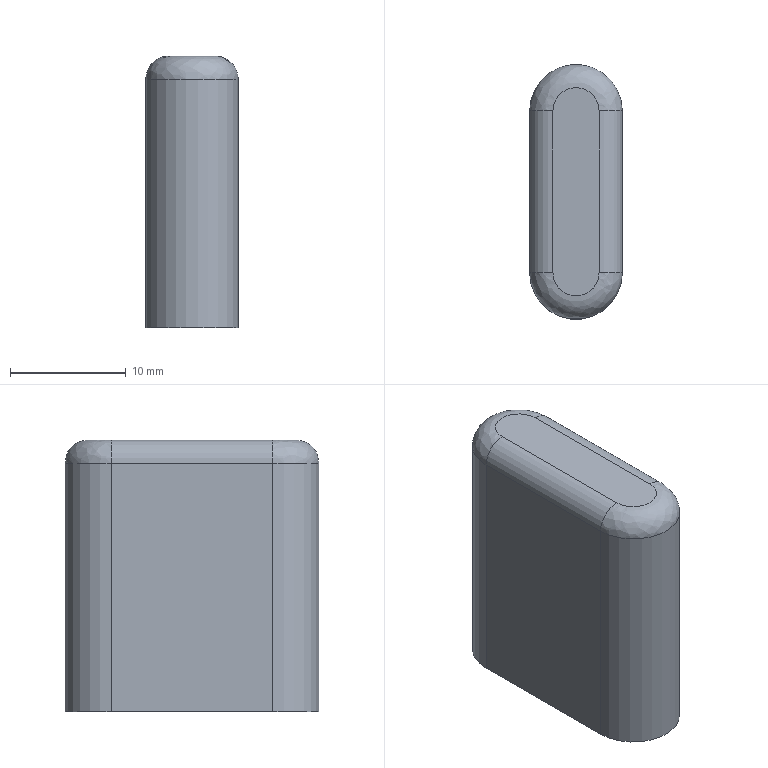Part | STEP file | Tube feed_id1790_x_t | 1 solid | 10 faces | box 8 x 22 x 23.5 mm | volume 3770 mm3 | plane 4 | cylinder 4 | spline 2 | commonest cylinder face diameters 4 x2 8 x2
STEP:
#1=CARTESIAN_POINT('',(0.,0.,0.));
#2=DIRECTION('',(0.,0.,1.));
#3=DIRECTION('',(1.,0.,0.));
#4=AXIS2_PLACEMENT_3D('',#1,#2,#3);
#5=CARTESIAN_POINT('',(17.,-36.964,-19.5));
#6=VERTEX_POINT('',#5);
#7=CARTESIAN_POINT('',(17.,-50.964,-19.5));
#8=VERTEX_POINT('',#7);
#9=CARTESIAN_POINT('',(17.,-32.964,-19.5));
#10=DIRECTION('',(0.,-1.,0.));
#11=VECTOR('',#10,1.);
#12=LINE('',#9,#11);
#13=CARTESIAN_POINT('',(25.,-32.964,-19.5));
#14=DIRECTION('',(0.,0.,-1.));
#15=DIRECTION('',(0.,-1.,0.));
#16=AXIS2_PLACEMENT_3D('',#13,#14,#15);
#17=PLANE('',#16);
#18=CARTESIAN_POINT('',(0.,8.));
#19=DIRECTION('',(1.,0.));
#20=VECTOR('',#19,1.);
#21=LINE('',#18,#20);
#22=(GEOMETRIC_REPRESENTATION_CONTEXT(2)PARAMETRIC_REPRESENTATION_CONTEXT()REPRESENTATION_CONTEXT('',''));
#23=DEFINITIONAL_REPRESENTATION('',(#21),#22);
#24=PCURVE('',#17,#23);
#25=CARTESIAN_POINT('',(17.,-32.964,-19.5));
#26=DIRECTION('',(1.,0.,0.));
#27=DIRECTION('',(0.,0.,-1.));
#28=AXIS2_PLACEMENT_3D('',#25,#26,#27);
#29=PLANE('',#28);
#30=CARTESIAN_POINT('',(0.,0.));
#31=DIRECTION('',(0.,-1.));
#32=VECTOR('',#31,1.);
#33=LINE('',#30,#32);
#34=(GEOMETRIC_REPRESENTATION_CONTEXT(2)PARAMETRIC_REPRESENTATION_CONTEXT()REPRESENTATION_CONTEXT('',''));
#35=DEFINITIONAL_REPRESENTATION('',(#33),#34);
#36=PCURVE('',#29,#35);
#37=SURFACE_CURVE('',#12,(#24,#36),.PCURVE_S1.);
#38=EDGE_CURVE('',#6,#8,#37,.T.);
#39=ORIENTED_EDGE('',*,*,#38,.F.);
#40=CARTESIAN_POINT('',(25.,-36.964,-19.5));
#41=VERTEX_POINT('',#40);
#42=CARTESIAN_POINT('',(21.,-36.964,-19.5));
#43=DIRECTION('',(0.,0.,1.));
#44=DIRECTION('',(0.,-1.,0.));
#45=AXIS2_PLACEMENT_3D('',#42,#43,#44);
#46=CIRCLE('',#45,4.);
#47=CARTESIAN_POINT('',(8.,4.));
#48=CARTESIAN_POINT('',(8.,-2.928));
#49=CARTESIAN_POINT('',(2.,0.5359));
#50=CARTESIAN_POINT('',(-4.,4.));
#51=CARTESIAN_POINT('',(2.,7.464));
#52=CARTESIAN_POINT('',(8.,10.928));
#53=CARTESIAN_POINT('',(8.,4.));
#54=(BOUNDED_CURVE()B_SPLINE_CURVE(2,(#47,#48,#49,#50,#51,#52,#53),.UNSPECIFIED.,.T.,.F.)B_SPLINE_CURVE_WITH_KNOTS((1,2,2,2,2,1),(-2.094,0.,2.094,4.189,6.283,8.378),.UNSPECIFIED.)CURVE()GEOMETRIC_REPRESENTATION_ITEM()RATIONAL_B_SPLINE_CURVE((1.,0.5,1.,0.5,1.,0.5,1.))REPRESENTATION_ITEM(''));
#55=(GEOMETRIC_REPRESENTATION_CONTEXT(2)PARAMETRIC_REPRESENTATION_CONTEXT()REPRESENTATION_CONTEXT('',''));
#56=DEFINITIONAL_REPRESENTATION('',(#54),#55);
#57=PCURVE('',#17,#56);
#58=CARTESIAN_POINT('',(21.,-36.964,-19.5));
#59=DIRECTION('',(0.,0.,-1.));
#60=DIRECTION('',(-1.,0.,0.));
#61=AXIS2_PLACEMENT_3D('',#58,#59,#60);
#62=CYLINDRICAL_SURFACE('',#61,4.);
#63=CARTESIAN_POINT('',(4.712,0.));
#64=DIRECTION('',(-1.,0.));
#65=VECTOR('',#64,1.);
#66=LINE('',#63,#65);
#67=(GEOMETRIC_REPRESENTATION_CONTEXT(2)PARAMETRIC_REPRESENTATION_CONTEXT()REPRESENTATION_CONTEXT('',''));
#68=DEFINITIONAL_REPRESENTATION('',(#66),#67);
#69=PCURVE('',#62,#68);
#70=SURFACE_CURVE('',#46,(#57,#69),.PCURVE_S1.);
#71=EDGE_CURVE('',#41,#6,#70,.T.);
#72=ORIENTED_EDGE('',*,*,#71,.F.);
#73=CARTESIAN_POINT('',(25.,-50.964,-19.5));
#74=VERTEX_POINT('',#73);
#75=CARTESIAN_POINT('',(25.,-32.964,-19.5));
#76=DIRECTION('',(0.,-1.,0.));
#77=VECTOR('',#76,1.);
#78=LINE('',#75,#77);
#79=CARTESIAN_POINT('',(0.,0.));
#80=DIRECTION('',(1.,0.));
#81=VECTOR('',#80,1.);
#82=LINE('',#79,#81);
#83=(GEOMETRIC_REPRESENTATION_CONTEXT(2)PARAMETRIC_REPRESENTATION_CONTEXT()REPRESENTATION_CONTEXT('',''));
#84=DEFINITIONAL_REPRESENTATION('',(#82),#83);
#85=PCURVE('',#17,#84);
#86=CARTESIAN_POINT('',(25.,-32.964,-19.5));
#87=DIRECTION('',(1.,0.,0.));
#88=DIRECTION('',(0.,0.,-1.));
#89=AXIS2_PLACEMENT_3D('',#86,#87,#88);
#90=PLANE('',#89);
#91=CARTESIAN_POINT('',(0.,0.));
#92=DIRECTION('',(0.,-1.));
#93=VECTOR('',#92,1.);
#94=LINE('',#91,#93);
#95=(GEOMETRIC_REPRESENTATION_CONTEXT(2)PARAMETRIC_REPRESENTATION_CONTEXT()REPRESENTATION_CONTEXT('',''));
#96=DEFINITIONAL_REPRESENTATION('',(#94),#95);
#97=PCURVE('',#90,#96);
#98=SURFACE_CURVE('',#78,(#85,#97),.PCURVE_S1.);
#99=EDGE_CURVE('',#41,#74,#98,.T.);
#100=ORIENTED_EDGE('',*,*,#99,.T.);
#101=CARTESIAN_POINT('',(21.,-50.964,-19.5));
#102=DIRECTION('',(0.,0.,1.));
#103=DIRECTION('',(0.,-1.,0.));
#104=AXIS2_PLACEMENT_3D('',#101,#102,#103);
#105=CIRCLE('',#104,4.);
#106=CARTESIAN_POINT('',(22.,4.));
#107=CARTESIAN_POINT('',(22.,-2.928));
#108=CARTESIAN_POINT('',(16.,0.5359));
#109=CARTESIAN_POINT('',(10.,4.));
#110=CARTESIAN_POINT('',(16.,7.464));
#111=CARTESIAN_POINT('',(22.,10.928));
#112=CARTESIAN_POINT('',(22.,4.));
#113=(BOUNDED_CURVE()B_SPLINE_CURVE(2,(#106,#107,#108,#109,#110,#111,#112),.UNSPECIFIED.,.T.,.F.)B_SPLINE_CURVE_WITH_KNOTS((1,2,2,2,2,1),(-2.094,0.,2.094,4.189,6.283,8.378),.UNSPECIFIED.)CURVE()GEOMETRIC_REPRESENTATION_ITEM()RATIONAL_B_SPLINE_CURVE((1.,0.5,1.,0.5,1.,0.5,1.))REPRESENTATION_ITEM(''));
#114=(GEOMETRIC_REPRESENTATION_CONTEXT(2)PARAMETRIC_REPRESENTATION_CONTEXT()REPRESENTATION_CONTEXT('',''));
#115=DEFINITIONAL_REPRESENTATION('',(#113),#114);
#116=PCURVE('',#17,#115);
#117=CARTESIAN_POINT('',(21.,-50.964,-19.5));
#118=DIRECTION('',(0.,0.,1.));
#119=DIRECTION('',(1.,0.,0.));
#120=AXIS2_PLACEMENT_3D('',#117,#118,#119);
#121=CYLINDRICAL_SURFACE('',#120,4.);
#122=CARTESIAN_POINT('',(-1.571,0.));
#123=DIRECTION('',(1.,0.));
#124=VECTOR('',#123,1.);
#125=LINE('',#122,#124);
#126=(GEOMETRIC_REPRESENTATION_CONTEXT(2)PARAMETRIC_REPRESENTATION_CONTEXT()REPRESENTATION_CONTEXT('',''));
#127=DEFINITIONAL_REPRESENTATION('',(#125),#126);
#128=PCURVE('',#121,#127);
#129=SURFACE_CURVE('',#105,(#116,#128),.PCURVE_S1.);
#130=EDGE_CURVE('',#8,#74,#129,.T.);
#131=ORIENTED_EDGE('',*,*,#130,.F.);
#132=EDGE_LOOP('',(#39,#72,#100,#131));
#133=FACE_BOUND('',#132,.T.);
#134=ADVANCED_FACE('',(#133),#17,.T.);
#135=CARTESIAN_POINT('',(19.,-50.964,4.));
#136=VERTEX_POINT('',#135);
#137=CARTESIAN_POINT('',(23.,-50.964,4.));
#138=VERTEX_POINT('',#137);
#139=CARTESIAN_POINT('',(21.,-50.964,4.));
#140=DIRECTION('',(0.,0.,1.));
#141=DIRECTION('',(0.,1.,0.));
#142=AXIS2_PLACEMENT_3D('',#139,#140,#141);
#143=CIRCLE('',#142,2.);
#144=CARTESIAN_POINT('',(25.,-32.964,4.));
#145=DIRECTION('',(0.,0.,-1.));
#146=DIRECTION('',(0.,-1.,0.));
#147=AXIS2_PLACEMENT_3D('',#144,#145,#146);
#148=PLANE('',#147);
#149=CARTESIAN_POINT('',(16.,4.));
#150=CARTESIAN_POINT('',(16.,7.464));
#151=CARTESIAN_POINT('',(19.,5.732));
#152=CARTESIAN_POINT('',(22.,4.));
#153=CARTESIAN_POINT('',(19.,2.268));
#154=CARTESIAN_POINT('',(16.,0.5359));
#155=CARTESIAN_POINT('',(16.,4.));
#156=(BOUNDED_CURVE()B_SPLINE_CURVE(2,(#149,#150,#151,#152,#153,#154,#155),.UNSPECIFIED.,.T.,.F.)B_SPLINE_CURVE_WITH_KNOTS((1,2,2,2,2,1),(-2.094,0.,2.094,4.189,6.283,8.378),.UNSPECIFIED.)CURVE()GEOMETRIC_REPRESENTATION_ITEM()RATIONAL_B_SPLINE_CURVE((1.,0.5,1.,0.5,1.,0.5,1.))REPRESENTATION_ITEM(''));
#157=(GEOMETRIC_REPRESENTATION_CONTEXT(2)PARAMETRIC_REPRESENTATION_CONTEXT()REPRESENTATION_CONTEXT('',''));
#158=DEFINITIONAL_REPRESENTATION('',(#156),#157);
#159=PCURVE('',#148,#158);
#160=CARTESIAN_POINT('',(25.,-50.964,2.));
#161=CARTESIAN_POINT('',(25.,-58.964,2.));
#162=CARTESIAN_POINT('',(17.,-58.964,2.));
#163=CARTESIAN_POINT('',(17.,-50.964,2.));
#164=CARTESIAN_POINT('',(25.,-50.964,3.172));
#165=CARTESIAN_POINT('',(25.,-58.964,3.172));
#166=CARTESIAN_POINT('',(17.,-58.964,3.172));
#167=CARTESIAN_POINT('',(17.,-50.964,3.172));
#168=CARTESIAN_POINT('',(24.172,-50.964,4.));
#169=CARTESIAN_POINT('',(24.172,-57.308,4.));
#170=CARTESIAN_POINT('',(17.828,-57.308,4.));
#171=CARTESIAN_POINT('',(17.828,-50.964,4.));
#172=CARTESIAN_POINT('',(23.,-50.964,4.));
#173=CARTESIAN_POINT('',(23.,-54.964,4.));
#174=CARTESIAN_POINT('',(19.,-54.964,4.));
#175=CARTESIAN_POINT('',(19.,-50.964,4.));
#176=(BOUNDED_SURFACE()B_SPLINE_SURFACE(3,3,((#160,#161,#162,#163),(#164,#165,#166,#167),(#168,#169,#170,#171),(#172,#173,#174,#175)),.UNSPECIFIED.,.F.,.F.,.F.)B_SPLINE_SURFACE_WITH_KNOTS((4,4),(4,4),(0.,1.),(0.,1.),.PIECEWISE_BEZIER_KNOTS.)GEOMETRIC_REPRESENTATION_ITEM()RATIONAL_B_SPLINE_SURFACE(((1.,0.3333,0.3333,1.),(0.8047,0.2682,0.2682,0.8047),(0.8047,0.2682,0.2682,0.8047),(1.,0.3333,0.3333,1.)))REPRESENTATION_ITEM('')SURFACE());
#177=CARTESIAN_POINT('',(1.,1.));
#178=CARTESIAN_POINT('',(1.,0.9763));
#179=CARTESIAN_POINT('',(1.,0.9319));
#180=CARTESIAN_POINT('',(1.,0.8733));
#181=CARTESIAN_POINT('',(1.,0.8206));
#182=CARTESIAN_POINT('',(1.,0.7724));
#183=CARTESIAN_POINT('',(1.,0.7279));
#184=CARTESIAN_POINT('',(1.,0.6861));
#185=CARTESIAN_POINT('',(1.,0.6465));
#186=CARTESIAN_POINT('',(1.,0.6086));
#187=CARTESIAN_POINT('',(1.,0.5718));
#188=CARTESIAN_POINT('',(1.,0.5357));
#189=CARTESIAN_POINT('',(1.,0.5));
#190=CARTESIAN_POINT('',(1.,0.4643));
#191=CARTESIAN_POINT('',(1.,0.4282));
#192=CARTESIAN_POINT('',(1.,0.3914));
#193=CARTESIAN_POINT('',(1.,0.3535));
#194=CARTESIAN_POINT('',(1.,0.3139));
#195=CARTESIAN_POINT('',(1.,0.2721));
#196=CARTESIAN_POINT('',(1.,0.2276));
#197=CARTESIAN_POINT('',(1.,0.1794));
#198=CARTESIAN_POINT('',(1.,0.1267));
#199=CARTESIAN_POINT('',(1.,0.06805));
#200=CARTESIAN_POINT('',(1.,0.02375));
#201=CARTESIAN_POINT('',(1.,0.));
#202=B_SPLINE_CURVE_WITH_KNOTS('',3,(#177,#178,#179,#180,#181,#182,#183,#184,#185,#186,#187,#188,#189,#190,#191,#192,#193,#194,#195,#196,#197,#198,#199,#200,#201),.UNSPECIFIED.,.F.,.F.,(4,1,1,1,1,1,1,1,1,1,1,1,1,1,1,1,1,1,1,1,1,1,4),(1.571,1.714,1.856,1.999,2.142,2.285,2.428,2.57,2.713,2.856,2.999,3.142,3.284,3.427,3.57,3.713,3.856,3.998,4.141,4.284,4.427,4.57,4.712),.QUASI_UNIFORM_KNOTS.);
#203=(GEOMETRIC_REPRESENTATION_CONTEXT(2)PARAMETRIC_REPRESENTATION_CONTEXT()REPRESENTATION_CONTEXT('',''));
#204=DEFINITIONAL_REPRESENTATION('',(#202),#203);
#205=PCURVE('',#176,#204);
#206=SURFACE_CURVE('',#143,(#159,#205),.PCURVE_S1.);
#207=EDGE_CURVE('',#136,#138,#206,.T.);
#208=ORIENTED_EDGE('',*,*,#207,.T.);
#209=CARTESIAN_POINT('',(23.,-36.964,4.));
#210=VERTEX_POINT('',#209);
#211=CARTESIAN_POINT('',(23.,-32.964,4.));
#212=DIRECTION('',(0.,1.,0.));
#213=VECTOR('',#212,1.);
#214=LINE('',#211,#213);
#215=CARTESIAN_POINT('',(0.,2.));
#216=DIRECTION('',(-1.,0.));
#217=VECTOR('',#216,1.);
#218=LINE('',#215,#217);
#219=(GEOMETRIC_REPRESENTATION_CONTEXT(2)PARAMETRIC_REPRESENTATION_CONTEXT()REPRESENTATION_CONTEXT('',''));
#220=DEFINITIONAL_REPRESENTATION('',(#218),#219);
#221=PCURVE('',#148,#220);
#222=CARTESIAN_POINT('',(23.,-32.964,2.));
#223=DIRECTION('',(0.,-1.,0.));
#224=DIRECTION('',(1.,0.,0.));
#225=AXIS2_PLACEMENT_3D('',#222,#223,#224);
#226=CYLINDRICAL_SURFACE('',#225,2.);
#227=CARTESIAN_POINT('',(1.571,0.));
#228=DIRECTION('',(0.,-1.));
#229=VECTOR('',#228,1.);
#230=LINE('',#227,#229);
#231=(GEOMETRIC_REPRESENTATION_CONTEXT(2)PARAMETRIC_REPRESENTATION_CONTEXT()REPRESENTATION_CONTEXT('',''));
#232=DEFINITIONAL_REPRESENTATION('',(#230),#231);
#233=PCURVE('',#226,#232);
#234=SURFACE_CURVE('',#214,(#221,#233),.PCURVE_S1.);
#235=EDGE_CURVE('',#138,#210,#234,.T.);
#236=ORIENTED_EDGE('',*,*,#235,.T.);
#237=CARTESIAN_POINT('',(19.,-36.964,4.));
#238=VERTEX_POINT('',#237);
#239=CARTESIAN_POINT('',(21.,-36.964,4.));
#240=DIRECTION('',(0.,0.,1.));
#241=DIRECTION('',(0.,1.,0.));
#242=AXIS2_PLACEMENT_3D('',#239,#240,#241);
#243=CIRCLE('',#242,2.);
#244=CARTESIAN_POINT('',(2.,4.));
#245=CARTESIAN_POINT('',(2.,7.464));
#246=CARTESIAN_POINT('',(5.,5.732));
#247=CARTESIAN_POINT('',(8.,4.));
#248=CARTESIAN_POINT('',(5.,2.268));
#249=CARTESIAN_POINT('',(2.,0.5359));
#250=CARTESIAN_POINT('',(2.,4.));
#251=(BOUNDED_CURVE()B_SPLINE_CURVE(2,(#244,#245,#246,#247,#248,#249,#250),.UNSPECIFIED.,.T.,.F.)B_SPLINE_CURVE_WITH_KNOTS((1,2,2,2,2,1),(-2.094,0.,2.094,4.189,6.283,8.378),.UNSPECIFIED.)CURVE()GEOMETRIC_REPRESENTATION_ITEM()RATIONAL_B_SPLINE_CURVE((1.,0.5,1.,0.5,1.,0.5,1.))REPRESENTATION_ITEM(''));
#252=(GEOMETRIC_REPRESENTATION_CONTEXT(2)PARAMETRIC_REPRESENTATION_CONTEXT()REPRESENTATION_CONTEXT('',''));
#253=DEFINITIONAL_REPRESENTATION('',(#251),#252);
#254=PCURVE('',#148,#253);
#255=CARTESIAN_POINT('',(17.,-36.964,2.));
#256=CARTESIAN_POINT('',(17.,-28.964,2.));
#257=CARTESIAN_POINT('',(25.,-28.964,2.));
#258=CARTESIAN_POINT('',(25.,-36.964,2.));
#259=CARTESIAN_POINT('',(17.,-36.964,3.172));
#260=CARTESIAN_POINT('',(17.,-28.964,3.172));
#261=CARTESIAN_POINT('',(25.,-28.964,3.172));
#262=CARTESIAN_POINT('',(25.,-36.964,3.172));
#263=CARTESIAN_POINT('',(17.828,-36.964,4.));
#264=CARTESIAN_POINT('',(17.828,-30.621,4.));
#265=CARTESIAN_POINT('',(24.172,-30.621,4.));
#266=CARTESIAN_POINT('',(24.172,-36.964,4.));
#267=CARTESIAN_POINT('',(19.,-36.964,4.));
#268=CARTESIAN_POINT('',(19.,-32.964,4.));
#269=CARTESIAN_POINT('',(23.,-32.964,4.));
#270=CARTESIAN_POINT('',(23.,-36.964,4.));
#271=(BOUNDED_SURFACE()B_SPLINE_SURFACE(3,3,((#255,#256,#257,#258),(#259,#260,#261,#262),(#263,#264,#265,#266),(#267,#268,#269,#270)),.UNSPECIFIED.,.F.,.F.,.F.)B_SPLINE_SURFACE_WITH_KNOTS((4,4),(4,4),(0.,1.),(0.,1.),.PIECEWISE_BEZIER_KNOTS.)GEOMETRIC_REPRESENTATION_ITEM()RATIONAL_B_SPLINE_SURFACE(((1.,0.3333,0.3333,1.),(0.8047,0.2682,0.2682,0.8047),(0.8047,0.2682,0.2682,0.8047),(1.,0.3333,0.3333,1.)))REPRESENTATION_ITEM('')SURFACE());
#272=CARTESIAN_POINT('',(1.,1.));
#273=CARTESIAN_POINT('',(1.,0.9763));
#274=CARTESIAN_POINT('',(1.,0.9319));
#275=CARTESIAN_POINT('',(1.,0.8733));
#276=CARTESIAN_POINT('',(1.,0.8206));
#277=CARTESIAN_POINT('',(1.,0.7724));
#278=CARTESIAN_POINT('',(1.,0.7279));
#279=CARTESIAN_POINT('',(1.,0.6861));
#280=CARTESIAN_POINT('',(1.,0.6465));
#281=CARTESIAN_POINT('',(1.,0.6086));
#282=CARTESIAN_POINT('',(1.,0.5718));
#283=CARTESIAN_POINT('',(1.,0.5357));
#284=CARTESIAN_POINT('',(1.,0.5));
#285=CARTESIAN_POINT('',(1.,0.4643));
#286=CARTESIAN_POINT('',(1.,0.4282));
#287=CARTESIAN_POINT('',(1.,0.3914));
#288=CARTESIAN_POINT('',(1.,0.3535));
#289=CARTESIAN_POINT('',(1.,0.3139));
#290=CARTESIAN_POINT('',(1.,0.2721));
#291=CARTESIAN_POINT('',(1.,0.2276));
#292=CARTESIAN_POINT('',(1.,0.1794));
#293=CARTESIAN_POINT('',(1.,0.1267));
#294=CARTESIAN_POINT('',(1.,0.06805));
#295=CARTESIAN_POINT('',(1.,0.02375));
#296=CARTESIAN_POINT('',(1.,0.));
#297=B_SPLINE_CURVE_WITH_KNOTS('',3,(#272,#273,#274,#275,#276,#277,#278,#279,#280,#281,#282,#283,#284,#285,#286,#287,#288,#289,#290,#291,#292,#293,#294,#295,#296),.UNSPECIFIED.,.F.,.F.,(4,1,1,1,1,1,1,1,1,1,1,1,1,1,1,1,1,1,1,1,1,1,4),(4.712,4.855,4.998,5.141,5.284,5.426,5.569,5.712,5.855,5.998,6.14,6.283,6.426,6.569,6.712,6.854,6.997,7.14,7.283,7.426,7.568,7.711,7.854),.QUASI_UNIFORM_KNOTS.);
#298=(GEOMETRIC_REPRESENTATION_CONTEXT(2)PARAMETRIC_REPRESENTATION_CONTEXT()REPRESENTATION_CONTEXT('',''));
#299=DEFINITIONAL_REPRESENTATION('',(#297),#298);
#300=PCURVE('',#271,#299);
#301=SURFACE_CURVE('',#243,(#254,#300),.PCURVE_S1.);
#302=EDGE_CURVE('',#210,#238,#301,.T.);
#303=ORIENTED_EDGE('',*,*,#302,.T.);
#304=CARTESIAN_POINT('',(19.,-50.964,4.));
#305=DIRECTION('',(0.,-1.,0.));
#306=VECTOR('',#305,1.);
#307=LINE('',#304,#306);
#308=CARTESIAN_POINT('',(18.,6.));
#309=DIRECTION('',(1.,0.));
#310=VECTOR('',#309,1.);
#311=LINE('',#308,#310);
#312=(GEOMETRIC_REPRESENTATION_CONTEXT(2)PARAMETRIC_REPRESENTATION_CONTEXT()REPRESENTATION_CONTEXT('',''));
#313=DEFINITIONAL_REPRESENTATION('',(#311),#312);
#314=PCURVE('',#148,#313);
#315=CARTESIAN_POINT('',(19.,-32.964,2.));
#316=DIRECTION('',(0.,1.,0.));
#317=DIRECTION('',(-1.,0.,0.));
#318=AXIS2_PLACEMENT_3D('',#315,#316,#317);
#319=CYLINDRICAL_SURFACE('',#318,2.);
#320=CARTESIAN_POINT('',(1.571,-18.));
#321=DIRECTION('',(0.,-1.));
#322=VECTOR('',#321,1.);
#323=LINE('',#320,#322);
#324=(GEOMETRIC_REPRESENTATION_CONTEXT(2)PARAMETRIC_REPRESENTATION_CONTEXT()REPRESENTATION_CONTEXT('',''));
#325=DEFINITIONAL_REPRESENTATION('',(#323),#324);
#326=PCURVE('',#319,#325);
#327=SURFACE_CURVE('',#307,(#314,#326),.PCURVE_S1.);
#328=EDGE_CURVE('',#238,#136,#327,.T.);
#329=ORIENTED_EDGE('',*,*,#328,.T.);
#330=EDGE_LOOP('',(#208,#236,#303,#329));
#331=FACE_BOUND('',#330,.T.);
#332=ADVANCED_FACE('',(#331),#148,.F.);
#333=CARTESIAN_POINT('',(17.,-50.964,2.));
#334=VERTEX_POINT('',#333);
#335=CARTESIAN_POINT('',(17.,-50.964,-19.5));
#336=DIRECTION('',(0.,0.,-1.));
#337=VECTOR('',#336,1.);
#338=LINE('',#335,#337);
#339=CARTESIAN_POINT('',(0.,-18.));
#340=DIRECTION('',(1.,0.));
#341=VECTOR('',#340,1.);
#342=LINE('',#339,#341);
#343=(GEOMETRIC_REPRESENTATION_CONTEXT(2)PARAMETRIC_REPRESENTATION_CONTEXT()REPRESENTATION_CONTEXT('',''));
#344=DEFINITIONAL_REPRESENTATION('',(#342),#343);
#345=PCURVE('',#29,#344);
#346=CARTESIAN_POINT('',(3.142,0.));
#347=DIRECTION('',(0.,-1.));
#348=VECTOR('',#347,1.);
#349=LINE('',#346,#348);
#350=(GEOMETRIC_REPRESENTATION_CONTEXT(2)PARAMETRIC_REPRESENTATION_CONTEXT()REPRESENTATION_CONTEXT('',''));
#351=DEFINITIONAL_REPRESENTATION('',(#349),#350);
#352=PCURVE('',#121,#351);
#353=SURFACE_CURVE('',#338,(#345,#352),.PCURVE_S1.);
#354=EDGE_CURVE('',#334,#8,#353,.T.);
#355=ORIENTED_EDGE('',*,*,#354,.F.);
#356=CARTESIAN_POINT('',(17.,-36.964,2.));
#357=VERTEX_POINT('',#356);
#358=CARTESIAN_POINT('',(17.,-36.964,2.));
#359=DIRECTION('',(0.,1.,0.));
#360=VECTOR('',#359,1.);
#361=LINE('',#358,#360);
#362=CARTESIAN_POINT('',(-21.5,-4.));
#363=DIRECTION('',(0.,1.));
#364=VECTOR('',#363,1.);
#365=LINE('',#362,#364);
#366=(GEOMETRIC_REPRESENTATION_CONTEXT(2)PARAMETRIC_REPRESENTATION_CONTEXT()REPRESENTATION_CONTEXT('',''));
#367=DEFINITIONAL_REPRESENTATION('',(#365),#366);
#368=PCURVE('',#29,#367);
#369=CARTESIAN_POINT('',(0.,-4.));
#370=DIRECTION('',(0.,1.));
#371=VECTOR('',#370,1.);
#372=LINE('',#369,#371);
#373=(GEOMETRIC_REPRESENTATION_CONTEXT(2)PARAMETRIC_REPRESENTATION_CONTEXT()REPRESENTATION_CONTEXT('',''));
#374=DEFINITIONAL_REPRESENTATION('',(#372),#373);
#375=PCURVE('',#319,#374);
#376=SURFACE_CURVE('',#361,(#368,#375),.PCURVE_S1.);
#377=EDGE_CURVE('',#334,#357,#376,.T.);
#378=ORIENTED_EDGE('',*,*,#377,.T.);
#379=CARTESIAN_POINT('',(17.,-36.964,4.));
#380=DIRECTION('',(0.,0.,1.));
#381=VECTOR('',#380,1.);
#382=LINE('',#379,#381);
#383=CARTESIAN_POINT('',(-23.5,-4.));
#384=DIRECTION('',(-1.,0.));
#385=VECTOR('',#384,1.);
#386=LINE('',#383,#385);
#387=(GEOMETRIC_REPRESENTATION_CONTEXT(2)PARAMETRIC_REPRESENTATION_CONTEXT()REPRESENTATION_CONTEXT('',''));
#388=DEFINITIONAL_REPRESENTATION('',(#386),#387);
#389=PCURVE('',#29,#388);
#390=CARTESIAN_POINT('',(0.,-23.5));
#391=DIRECTION('',(0.,-1.));
#392=VECTOR('',#391,1.);
#393=LINE('',#390,#392);
#394=(GEOMETRIC_REPRESENTATION_CONTEXT(2)PARAMETRIC_REPRESENTATION_CONTEXT()REPRESENTATION_CONTEXT('',''));
#395=DEFINITIONAL_REPRESENTATION('',(#393),#394);
#396=PCURVE('',#62,#395);
#397=SURFACE_CURVE('',#382,(#389,#396),.PCURVE_S1.);
#398=EDGE_CURVE('',#6,#357,#397,.T.);
#399=ORIENTED_EDGE('',*,*,#398,.F.);
#400=ORIENTED_EDGE('',*,*,#38,.T.);
#401=EDGE_LOOP('',(#355,#378,#399,#400));
#402=FACE_BOUND('',#401,.T.);
#403=ADVANCED_FACE('',(#402),#29,.F.);
#404=CARTESIAN_POINT('',(25.,-36.964,2.));
#405=VERTEX_POINT('',#404);
#406=CARTESIAN_POINT('',(25.,-36.964,-19.5));
#407=DIRECTION('',(0.,0.,-1.));
#408=VECTOR('',#407,1.);
#409=LINE('',#406,#408);
#410=CARTESIAN_POINT('',(0.,-4.));
#411=DIRECTION('',(1.,0.));
#412=VECTOR('',#411,1.);
#413=LINE('',#410,#412);
#414=(GEOMETRIC_REPRESENTATION_CONTEXT(2)PARAMETRIC_REPRESENTATION_CONTEXT()REPRESENTATION_CONTEXT('',''));
#415=DEFINITIONAL_REPRESENTATION('',(#413),#414);
#416=PCURVE('',#90,#415);
#417=CARTESIAN_POINT('',(3.142,0.));
#418=DIRECTION('',(0.,1.));
#419=VECTOR('',#418,1.);
#420=LINE('',#417,#419);
#421=(GEOMETRIC_REPRESENTATION_CONTEXT(2)PARAMETRIC_REPRESENTATION_CONTEXT()REPRESENTATION_CONTEXT('',''));
#422=DEFINITIONAL_REPRESENTATION('',(#420),#421);
#423=PCURVE('',#62,#422);
#424=SURFACE_CURVE('',#409,(#416,#423),.PCURVE_S1.);
#425=EDGE_CURVE('',#405,#41,#424,.T.);
#426=ORIENTED_EDGE('',*,*,#425,.F.);
#427=CARTESIAN_POINT('',(25.,-50.964,2.));
#428=VERTEX_POINT('',#427);
#429=CARTESIAN_POINT('',(25.,-32.964,2.));
#430=DIRECTION('',(0.,-1.,0.));
#431=VECTOR('',#430,1.);
#432=LINE('',#429,#431);
#433=CARTESIAN_POINT('',(-21.5,0.));
#434=DIRECTION('',(0.,-1.));
#435=VECTOR('',#434,1.);
#436=LINE('',#433,#435);
#437=(GEOMETRIC_REPRESENTATION_CONTEXT(2)PARAMETRIC_REPRESENTATION_CONTEXT()REPRESENTATION_CONTEXT('',''));
#438=DEFINITIONAL_REPRESENTATION('',(#436),#437);
#439=PCURVE('',#90,#438);
#440=CARTESIAN_POINT('',(0.,0.));
#441=DIRECTION('',(0.,1.));
#442=VECTOR('',#441,1.);
#443=LINE('',#440,#442);
#444=(GEOMETRIC_REPRESENTATION_CONTEXT(2)PARAMETRIC_REPRESENTATION_CONTEXT()REPRESENTATION_CONTEXT('',''));
#445=DEFINITIONAL_REPRESENTATION('',(#443),#444);
#446=PCURVE('',#226,#445);
#447=SURFACE_CURVE('',#432,(#439,#446),.PCURVE_S1.);
#448=EDGE_CURVE('',#405,#428,#447,.T.);
#449=ORIENTED_EDGE('',*,*,#448,.T.);
#450=CARTESIAN_POINT('',(25.,-50.964,-19.5));
#451=DIRECTION('',(0.,0.,1.));
#452=VECTOR('',#451,1.);
#453=LINE('',#450,#452);
#454=CARTESIAN_POINT('',(0.,-18.));
#455=DIRECTION('',(-1.,0.));
#456=VECTOR('',#455,1.);
#457=LINE('',#454,#456);
#458=(GEOMETRIC_REPRESENTATION_CONTEXT(2)PARAMETRIC_REPRESENTATION_CONTEXT()REPRESENTATION_CONTEXT('',''));
#459=DEFINITIONAL_REPRESENTATION('',(#457),#458);
#460=PCURVE('',#90,#459);
#461=CARTESIAN_POINT('',(6.283,0.));
#462=DIRECTION('',(0.,1.));
#463=VECTOR('',#462,1.);
#464=LINE('',#461,#463);
#465=(GEOMETRIC_REPRESENTATION_CONTEXT(2)PARAMETRIC_REPRESENTATION_CONTEXT()REPRESENTATION_CONTEXT('',''));
#466=DEFINITIONAL_REPRESENTATION('',(#464),#465);
#467=PCURVE('',#121,#466);
#468=SURFACE_CURVE('',#453,(#460,#467),.PCURVE_S1.);
#469=EDGE_CURVE('',#74,#428,#468,.T.);
#470=ORIENTED_EDGE('',*,*,#469,.F.);
#471=ORIENTED_EDGE('',*,*,#99,.F.);
#472=EDGE_LOOP('',(#426,#449,#470,#471));
#473=FACE_BOUND('',#472,.T.);
#474=ADVANCED_FACE('',(#473),#90,.T.);
#475=ORIENTED_EDGE('',*,*,#469,.T.);
#476=CARTESIAN_POINT('',(21.,-50.964,2.));
#477=DIRECTION('',(0.,0.,-1.));
#478=DIRECTION('',(0.,1.,0.));
#479=AXIS2_PLACEMENT_3D('',#476,#477,#478);
#480=CIRCLE('',#479,4.);
#481=CARTESIAN_POINT('',(7.854,21.5));
#482=DIRECTION('',(-1.,0.));
#483=VECTOR('',#482,1.);
#484=LINE('',#481,#483);
#485=(GEOMETRIC_REPRESENTATION_CONTEXT(2)PARAMETRIC_REPRESENTATION_CONTEXT()REPRESENTATION_CONTEXT('',''));
#486=DEFINITIONAL_REPRESENTATION('',(#484),#485);
#487=PCURVE('',#121,#486);
#488=CARTESIAN_POINT('',(0.,0.));
#489=CARTESIAN_POINT('',(0.,0.02375));
#490=CARTESIAN_POINT('',(0.,0.06805));
#491=CARTESIAN_POINT('',(0.,0.1267));
#492=CARTESIAN_POINT('',(0.,0.1794));
#493=CARTESIAN_POINT('',(0.,0.2276));
#494=CARTESIAN_POINT('',(0.,0.2721));
#495=CARTESIAN_POINT('',(0.,0.3139));
#496=CARTESIAN_POINT('',(0.,0.3535));
#497=CARTESIAN_POINT('',(0.,0.3914));
#498=CARTESIAN_POINT('',(0.,0.4282));
#499=CARTESIAN_POINT('',(0.,0.4643));
#500=CARTESIAN_POINT('',(0.,0.5));
#501=CARTESIAN_POINT('',(0.,0.5357));
#502=CARTESIAN_POINT('',(0.,0.5718));
#503=CARTESIAN_POINT('',(0.,0.6086));
#504=CARTESIAN_POINT('',(0.,0.6465));
#505=CARTESIAN_POINT('',(0.,0.6861));
#506=CARTESIAN_POINT('',(0.,0.7279));
#507=CARTESIAN_POINT('',(0.,0.7724));
#508=CARTESIAN_POINT('',(0.,0.8206));
#509=CARTESIAN_POINT('',(0.,0.8733));
#510=CARTESIAN_POINT('',(0.,0.9319));
#511=CARTESIAN_POINT('',(0.,0.9763));
#512=CARTESIAN_POINT('',(0.,1.));
#513=B_SPLINE_CURVE_WITH_KNOTS('',3,(#488,#489,#490,#491,#492,#493,#494,#495,#496,#497,#498,#499,#500,#501,#502,#503,#504,#505,#506,#507,#508,#509,#510,#511,#512),.UNSPECIFIED.,.F.,.F.,(4,1,1,1,1,1,1,1,1,1,1,1,1,1,1,1,1,1,1,1,1,1,4),(1.571,1.714,1.856,1.999,2.142,2.285,2.428,2.57,2.713,2.856,2.999,3.142,3.284,3.427,3.57,3.713,3.856,3.998,4.141,4.284,4.427,4.57,4.712),.QUASI_UNIFORM_KNOTS.);
#514=(GEOMETRIC_REPRESENTATION_CONTEXT(2)PARAMETRIC_REPRESENTATION_CONTEXT()REPRESENTATION_CONTEXT('',''));
#515=DEFINITIONAL_REPRESENTATION('',(#513),#514);
#516=PCURVE('',#176,#515);
#517=SURFACE_CURVE('',#480,(#487,#516),.PCURVE_S1.);
#518=EDGE_CURVE('',#428,#334,#517,.T.);
#519=ORIENTED_EDGE('',*,*,#518,.T.);
#520=ORIENTED_EDGE('',*,*,#354,.T.);
#521=ORIENTED_EDGE('',*,*,#130,.T.);
#522=EDGE_LOOP('',(#475,#519,#520,#521));
#523=FACE_BOUND('',#522,.T.);
#524=ADVANCED_FACE('',(#523),#121,.T.);
#525=ORIENTED_EDGE('',*,*,#398,.T.);
#526=CARTESIAN_POINT('',(21.,-36.964,2.));
#527=DIRECTION('',(0.,0.,-1.));
#528=DIRECTION('',(0.,1.,0.));
#529=AXIS2_PLACEMENT_3D('',#526,#527,#528);
#530=CIRCLE('',#529,4.);
#531=CARTESIAN_POINT('',(-4.712,-21.5));
#532=DIRECTION('',(1.,0.));
#533=VECTOR('',#532,1.);
#534=LINE('',#531,#533);
#535=(GEOMETRIC_REPRESENTATION_CONTEXT(2)PARAMETRIC_REPRESENTATION_CONTEXT()REPRESENTATION_CONTEXT('',''));
#536=DEFINITIONAL_REPRESENTATION('',(#534),#535);
#537=PCURVE('',#62,#536);
#538=CARTESIAN_POINT('',(0.,0.));
#539=CARTESIAN_POINT('',(0.,0.02375));
#540=CARTESIAN_POINT('',(0.,0.06805));
#541=CARTESIAN_POINT('',(0.,0.1267));
#542=CARTESIAN_POINT('',(0.,0.1794));
#543=CARTESIAN_POINT('',(0.,0.2276));
#544=CARTESIAN_POINT('',(0.,0.2721));
#545=CARTESIAN_POINT('',(0.,0.3139));
#546=CARTESIAN_POINT('',(0.,0.3535));
#547=CARTESIAN_POINT('',(0.,0.3914));
#548=CARTESIAN_POINT('',(0.,0.4282));
#549=CARTESIAN_POINT('',(0.,0.4643));
#550=CARTESIAN_POINT('',(0.,0.5));
#551=CARTESIAN_POINT('',(0.,0.5357));
#552=CARTESIAN_POINT('',(0.,0.5718));
#553=CARTESIAN_POINT('',(0.,0.6086));
#554=CARTESIAN_POINT('',(0.,0.6465));
#555=CARTESIAN_POINT('',(0.,0.6861));
#556=CARTESIAN_POINT('',(0.,0.7279));
#557=CARTESIAN_POINT('',(0.,0.7724));
#558=CARTESIAN_POINT('',(0.,0.8206));
#559=CARTESIAN_POINT('',(0.,0.8733));
#560=CARTESIAN_POINT('',(0.,0.9319));
#561=CARTESIAN_POINT('',(0.,0.9763));
#562=CARTESIAN_POINT('',(0.,1.));
#563=B_SPLINE_CURVE_WITH_KNOTS('',3,(#538,#539,#540,#541,#542,#543,#544,#545,#546,#547,#548,#549,#550,#551,#552,#553,#554,#555,#556,#557,#558,#559,#560,#561,#562),.UNSPECIFIED.,.F.,.F.,(4,1,1,1,1,1,1,1,1,1,1,1,1,1,1,1,1,1,1,1,1,1,4),(4.712,4.855,4.998,5.141,5.284,5.426,5.569,5.712,5.855,5.998,6.14,6.283,6.426,6.569,6.712,6.854,6.997,7.14,7.283,7.426,7.568,7.711,7.854),.QUASI_UNIFORM_KNOTS.);
#564=(GEOMETRIC_REPRESENTATION_CONTEXT(2)PARAMETRIC_REPRESENTATION_CONTEXT()REPRESENTATION_CONTEXT('',''));
#565=DEFINITIONAL_REPRESENTATION('',(#563),#564);
#566=PCURVE('',#271,#565);
#567=SURFACE_CURVE('',#530,(#537,#566),.PCURVE_S1.);
#568=EDGE_CURVE('',#357,#405,#567,.T.);
#569=ORIENTED_EDGE('',*,*,#568,.T.);
#570=ORIENTED_EDGE('',*,*,#425,.T.);
#571=ORIENTED_EDGE('',*,*,#71,.T.);
#572=EDGE_LOOP('',(#525,#569,#570,#571));
#573=FACE_BOUND('',#572,.T.);
#574=ADVANCED_FACE('',(#573),#62,.T.);
#575=CARTESIAN_POINT('',(19.,-36.964,2.));
#576=DIRECTION('',(0.,1.,0.));
#577=DIRECTION('',(0.,0.,1.));
#578=AXIS2_PLACEMENT_3D('',#575,#576,#577);
#579=CIRCLE('',#578,2.);
#580=CARTESIAN_POINT('',(-4.712,-4.));
#581=DIRECTION('',(1.,0.));
#582=VECTOR('',#581,1.);
#583=LINE('',#580,#582);
#584=(GEOMETRIC_REPRESENTATION_CONTEXT(2)PARAMETRIC_REPRESENTATION_CONTEXT()REPRESENTATION_CONTEXT('',''));
#585=DEFINITIONAL_REPRESENTATION('',(#583),#584);
#586=PCURVE('',#319,#585);
#587=CARTESIAN_POINT('',(0.,0.));
#588=CARTESIAN_POINT('',(0.01683,0.));
#589=CARTESIAN_POINT('',(0.04999,0.));
#590=CARTESIAN_POINT('',(0.09843,0.));
#591=CARTESIAN_POINT('',(0.1457,0.));
#592=CARTESIAN_POINT('',(0.192,0.));
#593=CARTESIAN_POINT('',(0.2375,0.));
#594=CARTESIAN_POINT('',(0.2823,0.));
#595=CARTESIAN_POINT('',(0.3265,0.));
#596=CARTESIAN_POINT('',(0.3703,0.));
#597=CARTESIAN_POINT('',(0.4137,0.));
#598=CARTESIAN_POINT('',(0.4569,0.));
#599=CARTESIAN_POINT('',(0.5,0.));
#600=CARTESIAN_POINT('',(0.5431,0.));
#601=CARTESIAN_POINT('',(0.5863,0.));
#602=CARTESIAN_POINT('',(0.6297,0.));
#603=CARTESIAN_POINT('',(0.6735,0.));
#604=CARTESIAN_POINT('',(0.7177,0.));
#605=CARTESIAN_POINT('',(0.7625,0.));
#606=CARTESIAN_POINT('',(0.808,0.));
#607=CARTESIAN_POINT('',(0.8543,0.));
#608=CARTESIAN_POINT('',(0.9016,0.));
#609=CARTESIAN_POINT('',(0.95,0.));
#610=CARTESIAN_POINT('',(0.9832,0.));
#611=CARTESIAN_POINT('',(1.,0.));
#612=B_SPLINE_CURVE_WITH_KNOTS('',3,(#587,#588,#589,#590,#591,#592,#593,#594,#595,#596,#597,#598,#599,#600,#601,#602,#603,#604,#605,#606,#607,#608,#609,#610,#611),.UNSPECIFIED.,.F.,.F.,(4,1,1,1,1,1,1,1,1,1,1,1,1,1,1,1,1,1,1,1,1,1,4),(4.712,4.784,4.855,4.927,4.998,5.069,5.141,5.212,5.284,5.355,5.426,5.498,5.569,5.641,5.712,5.783,5.855,5.926,5.998,6.069,6.14,6.212,6.283),.QUASI_UNIFORM_KNOTS.);
#613=(GEOMETRIC_REPRESENTATION_CONTEXT(2)PARAMETRIC_REPRESENTATION_CONTEXT()REPRESENTATION_CONTEXT('',''));
#614=DEFINITIONAL_REPRESENTATION('',(#612),#613);
#615=PCURVE('',#271,#614);
#616=SURFACE_CURVE('',#579,(#586,#615),.PCURVE_S1.);
#617=EDGE_CURVE('',#357,#238,#616,.T.);
#618=ORIENTED_EDGE('',*,*,#617,.F.);
#619=ORIENTED_EDGE('',*,*,#377,.F.);
#620=CARTESIAN_POINT('',(19.,-50.964,2.));
#621=DIRECTION('',(0.,-1.,0.));
#622=DIRECTION('',(0.,0.,-1.));
#623=AXIS2_PLACEMENT_3D('',#620,#621,#622);
#624=CIRCLE('',#623,2.);
#625=CARTESIAN_POINT('',(4.712,-18.));
#626=DIRECTION('',(-1.,0.));
#627=VECTOR('',#626,1.);
#628=LINE('',#625,#627);
#629=(GEOMETRIC_REPRESENTATION_CONTEXT(2)PARAMETRIC_REPRESENTATION_CONTEXT()REPRESENTATION_CONTEXT('',''));
#630=DEFINITIONAL_REPRESENTATION('',(#628),#629);
#631=PCURVE('',#319,#630);
#632=CARTESIAN_POINT('',(1.,1.));
#633=CARTESIAN_POINT('',(0.9832,1.));
#634=CARTESIAN_POINT('',(0.95,1.));
#635=CARTESIAN_POINT('',(0.9016,1.));
#636=CARTESIAN_POINT('',(0.8543,1.));
#637=CARTESIAN_POINT('',(0.808,1.));
#638=CARTESIAN_POINT('',(0.7625,1.));
#639=CARTESIAN_POINT('',(0.7177,1.));
#640=CARTESIAN_POINT('',(0.6735,1.));
#641=CARTESIAN_POINT('',(0.6297,1.));
#642=CARTESIAN_POINT('',(0.5863,1.));
#643=CARTESIAN_POINT('',(0.5431,1.));
#644=CARTESIAN_POINT('',(0.5,1.));
#645=CARTESIAN_POINT('',(0.4569,1.));
#646=CARTESIAN_POINT('',(0.4137,1.));
#647=CARTESIAN_POINT('',(0.3703,1.));
#648=CARTESIAN_POINT('',(0.3265,1.));
#649=CARTESIAN_POINT('',(0.2823,1.));
#650=CARTESIAN_POINT('',(0.2375,1.));
#651=CARTESIAN_POINT('',(0.192,1.));
#652=CARTESIAN_POINT('',(0.1457,1.));
#653=CARTESIAN_POINT('',(0.09843,1.));
#654=CARTESIAN_POINT('',(0.04999,1.));
#655=CARTESIAN_POINT('',(0.01683,1.));
#656=CARTESIAN_POINT('',(0.,1.));
#657=B_SPLINE_CURVE_WITH_KNOTS('',3,(#632,#633,#634,#635,#636,#637,#638,#639,#640,#641,#642,#643,#644,#645,#646,#647,#648,#649,#650,#651,#652,#653,#654,#655,#656),.UNSPECIFIED.,.F.,.F.,(4,1,1,1,1,1,1,1,1,1,1,1,1,1,1,1,1,1,1,1,1,1,4),(3.142,3.213,3.284,3.356,3.427,3.499,3.57,3.641,3.713,3.784,3.856,3.927,3.998,4.07,4.141,4.213,4.284,4.355,4.427,4.498,4.57,4.641,4.712),.QUASI_UNIFORM_KNOTS.);
#658=(GEOMETRIC_REPRESENTATION_CONTEXT(2)PARAMETRIC_REPRESENTATION_CONTEXT()REPRESENTATION_CONTEXT('',''));
#659=DEFINITIONAL_REPRESENTATION('',(#657),#658);
#660=PCURVE('',#176,#659);
#661=SURFACE_CURVE('',#624,(#631,#660),.PCURVE_S1.);
#662=EDGE_CURVE('',#136,#334,#661,.T.);
#663=ORIENTED_EDGE('',*,*,#662,.F.);
#664=ORIENTED_EDGE('',*,*,#328,.F.);
#665=EDGE_LOOP('',(#618,#619,#663,#664));
#666=FACE_BOUND('',#665,.T.);
#667=ADVANCED_FACE('',(#666),#319,.T.);
#668=ORIENTED_EDGE('',*,*,#662,.T.);
#669=ORIENTED_EDGE('',*,*,#518,.F.);
#670=CARTESIAN_POINT('',(23.,-50.964,2.));
#671=DIRECTION('',(0.,1.,0.));
#672=DIRECTION('',(0.,0.,1.));
#673=AXIS2_PLACEMENT_3D('',#670,#671,#672);
#674=CIRCLE('',#673,2.);
#675=CARTESIAN_POINT('',(1.,0.));
#676=CARTESIAN_POINT('',(0.9832,0.));
#677=CARTESIAN_POINT('',(0.95,0.));
#678=CARTESIAN_POINT('',(0.9016,0.));
#679=CARTESIAN_POINT('',(0.8543,0.));
#680=CARTESIAN_POINT('',(0.808,0.));
#681=CARTESIAN_POINT('',(0.7625,0.));
#682=CARTESIAN_POINT('',(0.7177,0.));
#683=CARTESIAN_POINT('',(0.6735,0.));
#684=CARTESIAN_POINT('',(0.6297,0.));
#685=CARTESIAN_POINT('',(0.5863,0.));
#686=CARTESIAN_POINT('',(0.5431,0.));
#687=CARTESIAN_POINT('',(0.5,0.));
#688=CARTESIAN_POINT('',(0.4569,0.));
#689=CARTESIAN_POINT('',(0.4137,0.));
#690=CARTESIAN_POINT('',(0.3703,0.));
#691=CARTESIAN_POINT('',(0.3265,0.));
#692=CARTESIAN_POINT('',(0.2823,0.));
#693=CARTESIAN_POINT('',(0.2375,0.));
#694=CARTESIAN_POINT('',(0.192,0.));
#695=CARTESIAN_POINT('',(0.1457,0.));
#696=CARTESIAN_POINT('',(0.09843,0.));
#697=CARTESIAN_POINT('',(0.04999,0.));
#698=CARTESIAN_POINT('',(0.01683,0.));
#699=CARTESIAN_POINT('',(0.,0.));
#700=B_SPLINE_CURVE_WITH_KNOTS('',3,(#675,#676,#677,#678,#679,#680,#681,#682,#683,#684,#685,#686,#687,#688,#689,#690,#691,#692,#693,#694,#695,#696,#697,#698,#699),.UNSPECIFIED.,.F.,.F.,(4,1,1,1,1,1,1,1,1,1,1,1,1,1,1,1,1,1,1,1,1,1,4),(0.,0.0714,0.1428,0.2142,0.2856,0.357,0.4284,0.4998,0.5712,0.6426,0.714,0.7854,0.8568,0.9282,0.9996,1.071,1.142,1.214,1.285,1.357,1.428,1.499,1.571),.QUASI_UNIFORM_KNOTS.);
#701=(GEOMETRIC_REPRESENTATION_CONTEXT(2)PARAMETRIC_REPRESENTATION_CONTEXT()REPRESENTATION_CONTEXT('',''));
#702=DEFINITIONAL_REPRESENTATION('',(#700),#701);
#703=PCURVE('',#176,#702);
#704=CARTESIAN_POINT('',(1.571,18.));
#705=DIRECTION('',(-1.,0.));
#706=VECTOR('',#705,1.);
#707=LINE('',#704,#706);
#708=(GEOMETRIC_REPRESENTATION_CONTEXT(2)PARAMETRIC_REPRESENTATION_CONTEXT()REPRESENTATION_CONTEXT('',''));
#709=DEFINITIONAL_REPRESENTATION('',(#707),#708);
#710=PCURVE('',#226,#709);
#711=SURFACE_CURVE('',#674,(#703,#710),.PCURVE_S1.);
#712=EDGE_CURVE('',#138,#428,#711,.T.);
#713=ORIENTED_EDGE('',*,*,#712,.F.);
#714=ORIENTED_EDGE('',*,*,#207,.F.);
#715=EDGE_LOOP('',(#668,#669,#713,#714));
#716=FACE_BOUND('',#715,.T.);
#717=ADVANCED_FACE('',(#716),#176,.T.);
#718=ORIENTED_EDGE('',*,*,#617,.T.);
#719=ORIENTED_EDGE('',*,*,#302,.F.);
#720=CARTESIAN_POINT('',(23.,-36.964,2.));
#721=DIRECTION('',(0.,-1.,0.));
#722=DIRECTION('',(0.,0.,-1.));
#723=AXIS2_PLACEMENT_3D('',#720,#721,#722);
#724=CIRCLE('',#723,2.);
#725=CARTESIAN_POINT('',(0.,1.));
#726=CARTESIAN_POINT('',(0.01683,1.));
#727=CARTESIAN_POINT('',(0.04999,1.));
#728=CARTESIAN_POINT('',(0.09843,1.));
#729=CARTESIAN_POINT('',(0.1457,1.));
#730=CARTESIAN_POINT('',(0.192,1.));
#731=CARTESIAN_POINT('',(0.2375,1.));
#732=CARTESIAN_POINT('',(0.2823,1.));
#733=CARTESIAN_POINT('',(0.3265,1.));
#734=CARTESIAN_POINT('',(0.3703,1.));
#735=CARTESIAN_POINT('',(0.4137,1.));
#736=CARTESIAN_POINT('',(0.4569,1.));
#737=CARTESIAN_POINT('',(0.5,1.));
#738=CARTESIAN_POINT('',(0.5431,1.));
#739=CARTESIAN_POINT('',(0.5863,1.));
#740=CARTESIAN_POINT('',(0.6297,1.));
#741=CARTESIAN_POINT('',(0.6735,1.));
#742=CARTESIAN_POINT('',(0.7177,1.));
#743=CARTESIAN_POINT('',(0.7625,1.));
#744=CARTESIAN_POINT('',(0.808,1.));
#745=CARTESIAN_POINT('',(0.8543,1.));
#746=CARTESIAN_POINT('',(0.9016,1.));
#747=CARTESIAN_POINT('',(0.95,1.));
#748=CARTESIAN_POINT('',(0.9832,1.));
#749=CARTESIAN_POINT('',(1.,1.));
#750=B_SPLINE_CURVE_WITH_KNOTS('',3,(#725,#726,#727,#728,#729,#730,#731,#732,#733,#734,#735,#736,#737,#738,#739,#740,#741,#742,#743,#744,#745,#746,#747,#748,#749),.UNSPECIFIED.,.F.,.F.,(4,1,1,1,1,1,1,1,1,1,1,1,1,1,1,1,1,1,1,1,1,1,4),(1.571,1.642,1.714,1.785,1.856,1.928,1.999,2.071,2.142,2.213,2.285,2.356,2.428,2.499,2.57,2.642,2.713,2.785,2.856,2.927,2.999,3.07,3.142),.QUASI_UNIFORM_KNOTS.);
#751=(GEOMETRIC_REPRESENTATION_CONTEXT(2)PARAMETRIC_REPRESENTATION_CONTEXT()REPRESENTATION_CONTEXT('',''));
#752=DEFINITIONAL_REPRESENTATION('',(#750),#751);
#753=PCURVE('',#271,#752);
#754=CARTESIAN_POINT('',(-1.571,4.));
#755=DIRECTION('',(1.,0.));
#756=VECTOR('',#755,1.);
#757=LINE('',#754,#756);
#758=(GEOMETRIC_REPRESENTATION_CONTEXT(2)PARAMETRIC_REPRESENTATION_CONTEXT()REPRESENTATION_CONTEXT('',''));
#759=DEFINITIONAL_REPRESENTATION('',(#757),#758);
#760=PCURVE('',#226,#759);
#761=SURFACE_CURVE('',#724,(#753,#760),.PCURVE_S1.);
#762=EDGE_CURVE('',#405,#210,#761,.T.);
#763=ORIENTED_EDGE('',*,*,#762,.F.);
#764=ORIENTED_EDGE('',*,*,#568,.F.);
#765=EDGE_LOOP('',(#718,#719,#763,#764));
#766=FACE_BOUND('',#765,.T.);
#767=ADVANCED_FACE('',(#766),#271,.T.);
#768=ORIENTED_EDGE('',*,*,#712,.T.);
#769=ORIENTED_EDGE('',*,*,#448,.F.);
#770=ORIENTED_EDGE('',*,*,#762,.T.);
#771=ORIENTED_EDGE('',*,*,#235,.F.);
#772=EDGE_LOOP('',(#768,#769,#770,#771));
#773=FACE_BOUND('',#772,.T.);
#774=ADVANCED_FACE('',(#773),#226,.T.);
#775=CLOSED_SHELL('',(#134,#332,#403,#474,#524,#574,#667,#717,#767,#774));
#776=MANIFOLD_SOLID_BREP('',#775);
#777=(LENGTH_UNIT()NAMED_UNIT(*)SI_UNIT(.MILLI.,.METRE.));
#778=UNCERTAINTY_MEASURE_WITH_UNIT(LENGTH_MEASURE(0.0000001),#777,'','');
#779=(NAMED_UNIT(*)PLANE_ANGLE_UNIT()SI_UNIT($,.RADIAN.));
#780=(NAMED_UNIT(*)SI_UNIT($,.STERADIAN.)SOLID_ANGLE_UNIT());
#781=(GEOMETRIC_REPRESENTATION_CONTEXT(3)GLOBAL_UNCERTAINTY_ASSIGNED_CONTEXT((#778))GLOBAL_UNIT_ASSIGNED_CONTEXT((#777,#779,#780))REPRESENTATION_CONTEXT('',''));
#782=ADVANCED_BREP_SHAPE_REPRESENTATION('',(#4,#776),#781);